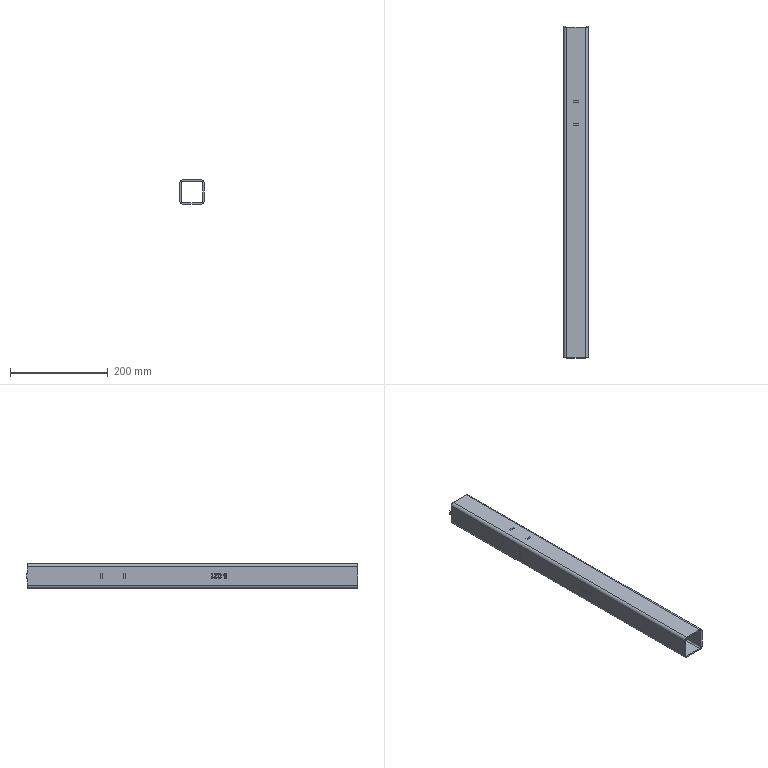Part | SolidWorks | features BaseBody 1 | 1 solid | 88 faces | box 50 x 679 x 50 mm | volume 365362 mm3 | plane 55 | spline 25 | cylinder 8 | commonest cylinder face diameters 6 x4 12 x4